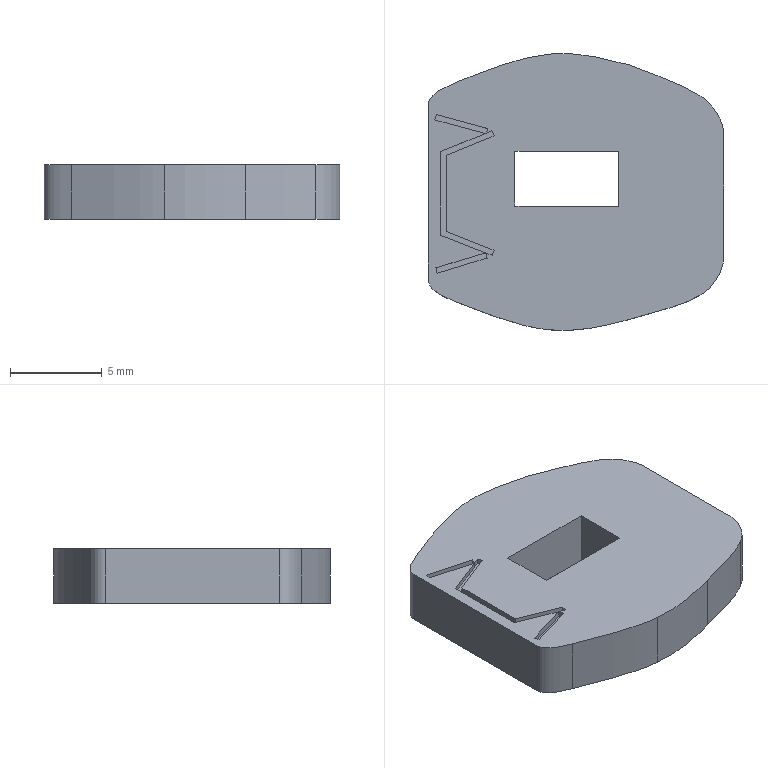Part | SolidWorks | features BaseBody 1 | 1 solid | 37 faces | box 16.136 x 15.14 x 3 mm | volume 585.362 mm3 | plane 26 | spline 11
STEP:
#1=CARTESIAN_POINT('',(-55.875,-105.115,1.2));
#2=VERTEX_POINT('',#1);
#3=CARTESIAN_POINT('',(-55.943,-105.364,1.2));
#4=VERTEX_POINT('',#3);
#5=CARTESIAN_POINT('',(-55.875,-105.115,1.2));
#6=DIRECTION('',(-0.2619,-0.9651,0.));
#7=VECTOR('',#6,1000.);
#8=LINE('',#5,#7);
#9=EDGE_CURVE('',#2,#4,#8,.T.);
#10=ORIENTED_EDGE('',*,*,#9,.F.);
#11=CARTESIAN_POINT('',(-58.677,-104.354,1.2));
#12=VERTEX_POINT('',#11);
#13=CARTESIAN_POINT('',(-55.875,-105.115,1.2));
#14=DIRECTION('',(-0.9651,0.2619,0.));
#15=VECTOR('',#14,1000.);
#16=LINE('',#13,#15);
#17=EDGE_CURVE('',#2,#12,#16,.T.);
#18=ORIENTED_EDGE('',*,*,#17,.T.);
#19=CARTESIAN_POINT('',(-58.755,-104.644,1.2));
#20=VERTEX_POINT('',#19);
#21=CARTESIAN_POINT('',(-58.755,-104.644,1.2));
#22=DIRECTION('',(0.2619,0.9651,0.));
#23=VECTOR('',#22,1000.);
#24=LINE('',#21,#23);
#25=EDGE_CURVE('',#20,#12,#24,.T.);
#26=ORIENTED_EDGE('',*,*,#25,.F.);
#27=CARTESIAN_POINT('',(-56.007,-105.39,1.2));
#28=VERTEX_POINT('',#27);
#29=CARTESIAN_POINT('',(-55.954,-105.404,1.2));
#30=DIRECTION('',(-0.9651,0.2619,0.));
#31=VECTOR('',#30,1000.);
#32=LINE('',#29,#31);
#33=EDGE_CURVE('',#28,#20,#32,.T.);
#34=ORIENTED_EDGE('',*,*,#33,.F.);
#35=CARTESIAN_POINT('',(-58.448,-106.374,1.2));
#36=VERTEX_POINT('',#35);
#37=CARTESIAN_POINT('',(-55.64,-105.242,1.2));
#38=DIRECTION('',(-0.9274,-0.3742,0.));
#39=VECTOR('',#38,1000.);
#40=LINE('',#37,#39);
#41=EDGE_CURVE('',#28,#36,#40,.T.);
#42=ORIENTED_EDGE('',*,*,#41,.T.);
#43=CARTESIAN_POINT('',(-58.448,-110.943,1.2));
#44=VERTEX_POINT('',#43);
#45=CARTESIAN_POINT('',(-58.448,-106.577,1.2));
#46=DIRECTION('',(0.,-1.,0.));
#47=VECTOR('',#46,1000.);
#48=LINE('',#45,#47);
#49=EDGE_CURVE('',#36,#44,#48,.T.);
#50=ORIENTED_EDGE('',*,*,#49,.T.);
#51=CARTESIAN_POINT('',(-55.637,-112.042,1.2));
#52=VERTEX_POINT('',#51);
#53=CARTESIAN_POINT('',(-58.257,-111.018,1.2));
#54=DIRECTION('',(0.9314,-0.3641,0.));
#55=VECTOR('',#54,1000.);
#56=LINE('',#53,#55);
#57=EDGE_CURVE('',#44,#52,#56,.T.);
#58=ORIENTED_EDGE('',*,*,#57,.T.);
#59=CARTESIAN_POINT('',(-55.528,-111.763,1.2));
#60=VERTEX_POINT('',#59);
#61=CARTESIAN_POINT('',(-55.528,-111.763,1.2));
#62=DIRECTION('',(-0.3641,-0.9314,0.));
#63=VECTOR('',#62,1000.);
#64=LINE('',#61,#63);
#65=EDGE_CURVE('',#60,#52,#64,.T.);
#66=ORIENTED_EDGE('',*,*,#65,.F.);
#67=CARTESIAN_POINT('',(-58.148,-110.738,1.2));
#68=VERTEX_POINT('',#67);
#69=CARTESIAN_POINT('',(-58.148,-110.738,1.2));
#70=DIRECTION('',(0.9314,-0.3641,0.));
#71=VECTOR('',#70,1000.);
#72=LINE('',#69,#71);
#73=EDGE_CURVE('',#68,#60,#72,.T.);
#74=ORIENTED_EDGE('',*,*,#73,.F.);
#75=CARTESIAN_POINT('',(-58.148,-106.577,1.2));
#76=VERTEX_POINT('',#75);
#77=CARTESIAN_POINT('',(-58.148,-106.577,1.2));
#78=DIRECTION('',(0.,-1.,0.));
#79=VECTOR('',#78,1000.);
#80=LINE('',#77,#79);
#81=EDGE_CURVE('',#76,#68,#80,.T.);
#82=ORIENTED_EDGE('',*,*,#81,.F.);
#83=CARTESIAN_POINT('',(-55.528,-105.52,1.2));
#84=VERTEX_POINT('',#83);
#85=CARTESIAN_POINT('',(-55.528,-105.52,1.2));
#86=DIRECTION('',(-0.9274,-0.3742,0.));
#87=VECTOR('',#86,1000.);
#88=LINE('',#85,#87);
#89=EDGE_CURVE('',#84,#76,#88,.T.);
#90=ORIENTED_EDGE('',*,*,#89,.F.);
#91=CARTESIAN_POINT('',(-55.64,-105.242,1.2));
#92=VERTEX_POINT('',#91);
#93=CARTESIAN_POINT('',(-55.64,-105.242,1.2));
#94=DIRECTION('',(0.3742,-0.9274,0.));
#95=VECTOR('',#94,1000.);
#96=LINE('',#93,#95);
#97=EDGE_CURVE('',#92,#84,#96,.T.);
#98=ORIENTED_EDGE('',*,*,#97,.F.);
#99=CARTESIAN_POINT('',(-55.64,-105.242,1.2));
#100=DIRECTION('',(-0.9274,-0.3742,0.));
#101=VECTOR('',#100,1000.);
#102=LINE('',#99,#101);
#103=EDGE_CURVE('',#92,#4,#102,.T.);
#104=ORIENTED_EDGE('',*,*,#103,.T.);
#105=EDGE_LOOP('',(#10,#18,#26,#34,#42,#50,#58,#66,#74,#82,#90,#98,#104));
#106=FACE_OUTER_BOUND('',#105,.T.);
#107=CARTESIAN_POINT('',(0.,0.,1.2));
#108=DIRECTION('',(0.,0.,-1.));
#109=DIRECTION('',(0.,-1.,0.));
#110=AXIS2_PLACEMENT_3D('',#107,#108,#109);
#111=PLANE('',#110);
#112=ADVANCED_FACE('',(#106),#111,.F.);
#113=CARTESIAN_POINT('',(-58.755,-104.644,1.5));
#114=VERTEX_POINT('',#113);
#115=CARTESIAN_POINT('',(-58.677,-104.354,1.5));
#116=VERTEX_POINT('',#115);
#117=CARTESIAN_POINT('',(-58.755,-104.644,1.5));
#118=DIRECTION('',(0.2619,0.9651,0.));
#119=VECTOR('',#118,1000.);
#120=LINE('',#117,#119);
#121=EDGE_CURVE('',#114,#116,#120,.T.);
#122=ORIENTED_EDGE('',*,*,#121,.F.);
#123=CARTESIAN_POINT('',(-58.755,-104.644,1.2));
#124=DIRECTION('',(0.,0.,1.));
#125=VECTOR('',#124,1000.);
#126=LINE('',#123,#125);
#127=EDGE_CURVE('',#20,#114,#126,.T.);
#128=ORIENTED_EDGE('',*,*,#127,.F.);
#129=ORIENTED_EDGE('',*,*,#25,.T.);
#130=CARTESIAN_POINT('',(-58.677,-104.354,1.2));
#131=DIRECTION('',(0.,0.,1.));
#132=VECTOR('',#131,1000.);
#133=LINE('',#130,#132);
#134=EDGE_CURVE('',#12,#116,#133,.T.);
#135=ORIENTED_EDGE('',*,*,#134,.T.);
#136=EDGE_LOOP('',(#122,#128,#129,#135));
#137=FACE_OUTER_BOUND('',#136,.T.);
#138=CARTESIAN_POINT('',(-58.755,-104.644,1.2));
#139=DIRECTION('',(0.9651,-0.2619,0.));
#140=DIRECTION('',(0.,0.,-1.));
#141=AXIS2_PLACEMENT_3D('',#138,#139,#140);
#142=PLANE('',#141);
#143=ADVANCED_FACE('',(#137),#142,.T.);
#144=CARTESIAN_POINT('',(-56.007,-105.39,1.5));
#145=VERTEX_POINT('',#144);
#146=CARTESIAN_POINT('',(-56.007,-105.39,1.2));
#147=DIRECTION('',(0.,0.,-1.));
#148=VECTOR('',#147,1000.);
#149=LINE('',#146,#148);
#150=EDGE_CURVE('',#145,#28,#149,.T.);
#151=ORIENTED_EDGE('',*,*,#150,.T.);
#152=ORIENTED_EDGE('',*,*,#33,.T.);
#153=ORIENTED_EDGE('',*,*,#127,.T.);
#154=CARTESIAN_POINT('',(-55.954,-105.404,1.5));
#155=DIRECTION('',(-0.9651,0.2619,0.));
#156=VECTOR('',#155,1000.);
#157=LINE('',#154,#156);
#158=EDGE_CURVE('',#145,#114,#157,.T.);
#159=ORIENTED_EDGE('',*,*,#158,.F.);
#160=EDGE_LOOP('',(#151,#152,#153,#159));
#161=FACE_OUTER_BOUND('',#160,.T.);
#162=CARTESIAN_POINT('',(-55.954,-105.404,1.2));
#163=DIRECTION('',(0.2619,0.9651,0.));
#164=DIRECTION('',(0.,0.,-1.));
#165=AXIS2_PLACEMENT_3D('',#162,#163,#164);
#166=PLANE('',#165);
#167=ADVANCED_FACE('',(#161),#166,.T.);
#168=CARTESIAN_POINT('',(-55.943,-105.364,1.5));
#169=VERTEX_POINT('',#168);
#170=CARTESIAN_POINT('',(-55.943,-105.364,1.2));
#171=DIRECTION('',(0.,0.,1.));
#172=VECTOR('',#171,1000.);
#173=LINE('',#170,#172);
#174=EDGE_CURVE('',#4,#169,#173,.T.);
#175=ORIENTED_EDGE('',*,*,#174,.T.);
#176=CARTESIAN_POINT('',(-55.875,-105.115,1.5));
#177=VERTEX_POINT('',#176);
#178=CARTESIAN_POINT('',(-55.875,-105.115,1.5));
#179=DIRECTION('',(-0.2619,-0.9651,0.));
#180=VECTOR('',#179,1000.);
#181=LINE('',#178,#180);
#182=EDGE_CURVE('',#177,#169,#181,.T.);
#183=ORIENTED_EDGE('',*,*,#182,.F.);
#184=CARTESIAN_POINT('',(-55.875,-105.115,1.2));
#185=DIRECTION('',(0.,0.,1.));
#186=VECTOR('',#185,1000.);
#187=LINE('',#184,#186);
#188=EDGE_CURVE('',#2,#177,#187,.T.);
#189=ORIENTED_EDGE('',*,*,#188,.F.);
#190=ORIENTED_EDGE('',*,*,#9,.T.);
#191=EDGE_LOOP('',(#175,#183,#189,#190));
#192=FACE_OUTER_BOUND('',#191,.T.);
#193=CARTESIAN_POINT('',(-55.875,-105.115,1.2));
#194=DIRECTION('',(-0.9651,0.2619,0.));
#195=DIRECTION('',(0.,0.,1.));
#196=AXIS2_PLACEMENT_3D('',#193,#194,#195);
#197=PLANE('',#196);
#198=ADVANCED_FACE('',(#192),#197,.T.);
#199=CARTESIAN_POINT('',(-55.875,-105.115,1.5));
#200=DIRECTION('',(-0.9651,0.2619,0.));
#201=VECTOR('',#200,1000.);
#202=LINE('',#199,#201);
#203=EDGE_CURVE('',#177,#116,#202,.T.);
#204=ORIENTED_EDGE('',*,*,#203,.T.);
#205=ORIENTED_EDGE('',*,*,#134,.F.);
#206=ORIENTED_EDGE('',*,*,#17,.F.);
#207=ORIENTED_EDGE('',*,*,#188,.T.);
#208=EDGE_LOOP('',(#204,#205,#206,#207));
#209=FACE_OUTER_BOUND('',#208,.T.);
#210=CARTESIAN_POINT('',(-55.875,-105.115,1.2));
#211=DIRECTION('',(0.2619,0.9651,0.));
#212=DIRECTION('',(0.,0.,-1.));
#213=AXIS2_PLACEMENT_3D('',#210,#211,#212);
#214=PLANE('',#213);
#215=ADVANCED_FACE('',(#209),#214,.F.);
#216=CARTESIAN_POINT('',(-58.448,-106.374,1.5));
#217=VERTEX_POINT('',#216);
#218=CARTESIAN_POINT('',(-55.64,-105.242,1.5));
#219=DIRECTION('',(-0.9274,-0.3742,0.));
#220=VECTOR('',#219,1000.);
#221=LINE('',#218,#220);
#222=EDGE_CURVE('',#145,#217,#221,.T.);
#223=ORIENTED_EDGE('',*,*,#222,.T.);
#224=CARTESIAN_POINT('',(-58.448,-106.374,1.2));
#225=DIRECTION('',(0.,0.,1.));
#226=VECTOR('',#225,1000.);
#227=LINE('',#224,#226);
#228=EDGE_CURVE('',#36,#217,#227,.T.);
#229=ORIENTED_EDGE('',*,*,#228,.F.);
#230=ORIENTED_EDGE('',*,*,#41,.F.);
#231=ORIENTED_EDGE('',*,*,#150,.F.);
#232=EDGE_LOOP('',(#223,#229,#230,#231));
#233=FACE_OUTER_BOUND('',#232,.T.);
#234=CARTESIAN_POINT('',(-55.64,-105.242,1.2));
#235=DIRECTION('',(-0.3742,0.9274,0.));
#236=DIRECTION('',(0.,0.,1.));
#237=AXIS2_PLACEMENT_3D('',#234,#235,#236);
#238=PLANE('',#237);
#239=ADVANCED_FACE('',(#233),#238,.F.);
#240=CARTESIAN_POINT('',(-58.448,-110.943,1.5));
#241=VERTEX_POINT('',#240);
#242=CARTESIAN_POINT('',(-58.448,-106.577,1.5));
#243=DIRECTION('',(0.,-1.,0.));
#244=VECTOR('',#243,1000.);
#245=LINE('',#242,#244);
#246=EDGE_CURVE('',#217,#241,#245,.T.);
#247=ORIENTED_EDGE('',*,*,#246,.T.);
#248=CARTESIAN_POINT('',(-58.448,-110.943,1.2));
#249=DIRECTION('',(0.,0.,1.));
#250=VECTOR('',#249,1000.);
#251=LINE('',#248,#250);
#252=EDGE_CURVE('',#44,#241,#251,.T.);
#253=ORIENTED_EDGE('',*,*,#252,.F.);
#254=ORIENTED_EDGE('',*,*,#49,.F.);
#255=ORIENTED_EDGE('',*,*,#228,.T.);
#256=EDGE_LOOP('',(#247,#253,#254,#255));
#257=FACE_OUTER_BOUND('',#256,.T.);
#258=CARTESIAN_POINT('',(-58.448,-106.577,1.2));
#259=DIRECTION('',(-1.,0.,0.));
#260=DIRECTION('',(0.,0.,1.));
#261=AXIS2_PLACEMENT_3D('',#258,#259,#260);
#262=PLANE('',#261);
#263=ADVANCED_FACE('',(#257),#262,.F.);
#264=CARTESIAN_POINT('',(-55.637,-112.042,1.5));
#265=VERTEX_POINT('',#264);
#266=CARTESIAN_POINT('',(-58.257,-111.018,1.5));
#267=DIRECTION('',(0.9314,-0.3641,0.));
#268=VECTOR('',#267,1000.);
#269=LINE('',#266,#268);
#270=EDGE_CURVE('',#241,#265,#269,.T.);
#271=ORIENTED_EDGE('',*,*,#270,.T.);
#272=CARTESIAN_POINT('',(-55.637,-112.042,1.2));
#273=DIRECTION('',(0.,0.,1.));
#274=VECTOR('',#273,1000.);
#275=LINE('',#272,#274);
#276=EDGE_CURVE('',#52,#265,#275,.T.);
#277=ORIENTED_EDGE('',*,*,#276,.F.);
#278=ORIENTED_EDGE('',*,*,#57,.F.);
#279=ORIENTED_EDGE('',*,*,#252,.T.);
#280=EDGE_LOOP('',(#271,#277,#278,#279));
#281=FACE_OUTER_BOUND('',#280,.T.);
#282=CARTESIAN_POINT('',(-58.257,-111.018,1.2));
#283=DIRECTION('',(-0.3641,-0.9314,0.));
#284=DIRECTION('',(-0.9314,0.3641,0.));
#285=AXIS2_PLACEMENT_3D('',#282,#283,#284);
#286=PLANE('',#285);
#287=ADVANCED_FACE('',(#281),#286,.F.);
#288=CARTESIAN_POINT('',(-55.528,-111.763,1.5));
#289=VERTEX_POINT('',#288);
#290=CARTESIAN_POINT('',(-55.528,-111.763,1.5));
#291=DIRECTION('',(-0.3641,-0.9314,0.));
#292=VECTOR('',#291,1000.);
#293=LINE('',#290,#292);
#294=EDGE_CURVE('',#289,#265,#293,.T.);
#295=ORIENTED_EDGE('',*,*,#294,.F.);
#296=CARTESIAN_POINT('',(-55.528,-111.763,1.2));
#297=DIRECTION('',(0.,0.,1.));
#298=VECTOR('',#297,1000.);
#299=LINE('',#296,#298);
#300=EDGE_CURVE('',#60,#289,#299,.T.);
#301=ORIENTED_EDGE('',*,*,#300,.F.);
#302=ORIENTED_EDGE('',*,*,#65,.T.);
#303=ORIENTED_EDGE('',*,*,#276,.T.);
#304=EDGE_LOOP('',(#295,#301,#302,#303));
#305=FACE_OUTER_BOUND('',#304,.T.);
#306=CARTESIAN_POINT('',(-55.528,-111.763,1.2));
#307=DIRECTION('',(-0.9314,0.3641,0.));
#308=DIRECTION('',(0.,0.,1.));
#309=AXIS2_PLACEMENT_3D('',#306,#307,#308);
#310=PLANE('',#309);
#311=ADVANCED_FACE('',(#305),#310,.T.);
#312=CARTESIAN_POINT('',(-58.148,-110.738,1.5));
#313=VERTEX_POINT('',#312);
#314=CARTESIAN_POINT('',(-58.148,-110.738,1.5));
#315=DIRECTION('',(0.9314,-0.3641,0.));
#316=VECTOR('',#315,1000.);
#317=LINE('',#314,#316);
#318=EDGE_CURVE('',#313,#289,#317,.T.);
#319=ORIENTED_EDGE('',*,*,#318,.F.);
#320=CARTESIAN_POINT('',(-58.148,-110.738,1.2));
#321=DIRECTION('',(0.,0.,1.));
#322=VECTOR('',#321,1000.);
#323=LINE('',#320,#322);
#324=EDGE_CURVE('',#68,#313,#323,.T.);
#325=ORIENTED_EDGE('',*,*,#324,.F.);
#326=ORIENTED_EDGE('',*,*,#73,.T.);
#327=ORIENTED_EDGE('',*,*,#300,.T.);
#328=EDGE_LOOP('',(#319,#325,#326,#327));
#329=FACE_OUTER_BOUND('',#328,.T.);
#330=CARTESIAN_POINT('',(-58.148,-110.738,1.2));
#331=DIRECTION('',(-0.3641,-0.9314,0.));
#332=DIRECTION('',(-0.9314,0.3641,0.));
#333=AXIS2_PLACEMENT_3D('',#330,#331,#332);
#334=PLANE('',#333);
#335=ADVANCED_FACE('',(#329),#334,.T.);
#336=CARTESIAN_POINT('',(-58.148,-106.577,1.5));
#337=VERTEX_POINT('',#336);
#338=CARTESIAN_POINT('',(-58.148,-106.577,1.5));
#339=DIRECTION('',(0.,-1.,0.));
#340=VECTOR('',#339,1000.);
#341=LINE('',#338,#340);
#342=EDGE_CURVE('',#337,#313,#341,.T.);
#343=ORIENTED_EDGE('',*,*,#342,.F.);
#344=CARTESIAN_POINT('',(-58.148,-106.577,1.2));
#345=DIRECTION('',(0.,0.,1.));
#346=VECTOR('',#345,1000.);
#347=LINE('',#344,#346);
#348=EDGE_CURVE('',#76,#337,#347,.T.);
#349=ORIENTED_EDGE('',*,*,#348,.F.);
#350=ORIENTED_EDGE('',*,*,#81,.T.);
#351=ORIENTED_EDGE('',*,*,#324,.T.);
#352=EDGE_LOOP('',(#343,#349,#350,#351));
#353=FACE_OUTER_BOUND('',#352,.T.);
#354=CARTESIAN_POINT('',(-58.148,-106.577,1.2));
#355=DIRECTION('',(-1.,0.,0.));
#356=DIRECTION('',(0.,0.,1.));
#357=AXIS2_PLACEMENT_3D('',#354,#355,#356);
#358=PLANE('',#357);
#359=ADVANCED_FACE('',(#353),#358,.T.);
#360=CARTESIAN_POINT('',(-55.528,-105.52,1.5));
#361=VERTEX_POINT('',#360);
#362=CARTESIAN_POINT('',(-55.528,-105.52,1.5));
#363=DIRECTION('',(-0.9274,-0.3742,0.));
#364=VECTOR('',#363,1000.);
#365=LINE('',#362,#364);
#366=EDGE_CURVE('',#361,#337,#365,.T.);
#367=ORIENTED_EDGE('',*,*,#366,.F.);
#368=CARTESIAN_POINT('',(-55.528,-105.52,1.2));
#369=DIRECTION('',(0.,0.,1.));
#370=VECTOR('',#369,1000.);
#371=LINE('',#368,#370);
#372=EDGE_CURVE('',#84,#361,#371,.T.);
#373=ORIENTED_EDGE('',*,*,#372,.F.);
#374=ORIENTED_EDGE('',*,*,#89,.T.);
#375=ORIENTED_EDGE('',*,*,#348,.T.);
#376=EDGE_LOOP('',(#367,#373,#374,#375));
#377=FACE_OUTER_BOUND('',#376,.T.);
#378=CARTESIAN_POINT('',(-55.528,-105.52,1.2));
#379=DIRECTION('',(-0.3742,0.9274,0.));
#380=DIRECTION('',(0.,0.,1.));
#381=AXIS2_PLACEMENT_3D('',#378,#379,#380);
#382=PLANE('',#381);
#383=ADVANCED_FACE('',(#377),#382,.T.);
#384=CARTESIAN_POINT('',(-55.64,-105.242,1.5));
#385=VERTEX_POINT('',#384);
#386=CARTESIAN_POINT('',(-55.64,-105.242,1.5));
#387=DIRECTION('',(0.3742,-0.9274,0.));
#388=VECTOR('',#387,1000.);
#389=LINE('',#386,#388);
#390=EDGE_CURVE('',#385,#361,#389,.T.);
#391=ORIENTED_EDGE('',*,*,#390,.F.);
#392=CARTESIAN_POINT('',(-55.64,-105.242,1.2));
#393=DIRECTION('',(0.,0.,1.));
#394=VECTOR('',#393,1000.);
#395=LINE('',#392,#394);
#396=EDGE_CURVE('',#92,#385,#395,.T.);
#397=ORIENTED_EDGE('',*,*,#396,.F.);
#398=ORIENTED_EDGE('',*,*,#97,.T.);
#399=ORIENTED_EDGE('',*,*,#372,.T.);
#400=EDGE_LOOP('',(#391,#397,#398,#399));
#401=FACE_OUTER_BOUND('',#400,.T.);
#402=CARTESIAN_POINT('',(-55.64,-105.242,1.2));
#403=DIRECTION('',(-0.9274,-0.3742,0.));
#404=DIRECTION('',(-0.3742,0.9274,0.));
#405=AXIS2_PLACEMENT_3D('',#402,#403,#404);
#406=PLANE('',#405);
#407=ADVANCED_FACE('',(#401),#406,.T.);
#408=ORIENTED_EDGE('',*,*,#103,.F.);
#409=ORIENTED_EDGE('',*,*,#396,.T.);
#410=CARTESIAN_POINT('',(-55.64,-105.242,1.5));
#411=DIRECTION('',(-0.9274,-0.3742,0.));
#412=VECTOR('',#411,1000.);
#413=LINE('',#410,#412);
#414=EDGE_CURVE('',#385,#169,#413,.T.);
#415=ORIENTED_EDGE('',*,*,#414,.T.);
#416=ORIENTED_EDGE('',*,*,#174,.F.);
#417=EDGE_LOOP('',(#408,#409,#415,#416));
#418=FACE_OUTER_BOUND('',#417,.T.);
#419=CARTESIAN_POINT('',(-55.64,-105.242,1.2));
#420=DIRECTION('',(-0.3742,0.9274,0.));
#421=DIRECTION('',(0.,0.,1.));
#422=AXIS2_PLACEMENT_3D('',#419,#420,#421);
#423=PLANE('',#422);
#424=ADVANCED_FACE('',(#418),#423,.F.);
#425=CARTESIAN_POINT('',(-58.627,-113.019,1.2));
#426=VERTEX_POINT('',#425);
#427=CARTESIAN_POINT('',(-55.905,-112.191,1.2));
#428=VERTEX_POINT('',#427);
#429=CARTESIAN_POINT('',(-58.627,-113.019,1.2));
#430=DIRECTION('',(0.9567,0.2911,0.));
#431=VECTOR('',#430,1000.);
#432=LINE('',#429,#431);
#433=EDGE_CURVE('',#426,#428,#432,.T.);
#434=ORIENTED_EDGE('',*,*,#433,.T.);
#435=CARTESIAN_POINT('',(-55.992,-111.904,1.2));
#436=VERTEX_POINT('',#435);
#437=CARTESIAN_POINT('',(-55.992,-111.904,1.2));
#438=DIRECTION('',(0.2911,-0.9567,0.));
#439=VECTOR('',#438,1000.);
#440=LINE('',#437,#439);
#441=EDGE_CURVE('',#436,#428,#440,.T.);
#442=ORIENTED_EDGE('',*,*,#441,.F.);
#443=CARTESIAN_POINT('',(-58.714,-112.732,1.2));
#444=VERTEX_POINT('',#443);
#445=CARTESIAN_POINT('',(-58.714,-112.732,1.2));
#446=DIRECTION('',(0.9567,0.2911,0.));
#447=VECTOR('',#446,1000.);
#448=LINE('',#445,#447);
#449=EDGE_CURVE('',#444,#436,#448,.T.);
#450=ORIENTED_EDGE('',*,*,#449,.F.);
#451=CARTESIAN_POINT('',(-58.627,-113.019,1.2));
#452=DIRECTION('',(-0.2911,0.9567,0.));
#453=VECTOR('',#452,1000.);
#454=LINE('',#451,#453);
#455=EDGE_CURVE('',#426,#444,#454,.T.);
#456=ORIENTED_EDGE('',*,*,#455,.F.);
#457=EDGE_LOOP('',(#434,#442,#450,#456));
#458=FACE_OUTER_BOUND('',#457,.T.);
#459=CARTESIAN_POINT('',(0.,0.,1.2));
#460=DIRECTION('',(0.,0.,-1.));
#461=DIRECTION('',(0.,-1.,0.));
#462=AXIS2_PLACEMENT_3D('',#459,#460,#461);
#463=PLANE('',#462);
#464=ADVANCED_FACE('',(#458),#463,.F.);
#465=CARTESIAN_POINT('',(-55.992,-111.904,1.5));
#466=VERTEX_POINT('',#465);
#467=CARTESIAN_POINT('',(-55.905,-112.191,1.5));
#468=VERTEX_POINT('',#467);
#469=CARTESIAN_POINT('',(-55.992,-111.904,1.5));
#470=DIRECTION('',(0.2911,-0.9567,0.));
#471=VECTOR('',#470,1000.);
#472=LINE('',#469,#471);
#473=EDGE_CURVE('',#466,#468,#472,.T.);
#474=ORIENTED_EDGE('',*,*,#473,.F.);
#475=CARTESIAN_POINT('',(-55.992,-111.904,1.2));
#476=DIRECTION('',(0.,0.,1.));
#477=VECTOR('',#476,1000.);
#478=LINE('',#475,#477);
#479=EDGE_CURVE('',#436,#466,#478,.T.);
#480=ORIENTED_EDGE('',*,*,#479,.F.);
#481=ORIENTED_EDGE('',*,*,#441,.T.);
#482=CARTESIAN_POINT('',(-55.905,-112.191,1.2));
#483=DIRECTION('',(0.,0.,1.));
#484=VECTOR('',#483,1000.);
#485=LINE('',#482,#484);
#486=EDGE_CURVE('',#428,#468,#485,.T.);
#487=ORIENTED_EDGE('',*,*,#486,.T.);
#488=EDGE_LOOP('',(#474,#480,#481,#487));
#489=FACE_OUTER_BOUND('',#488,.T.);
#490=CARTESIAN_POINT('',(-55.992,-111.904,1.2));
#491=DIRECTION('',(-0.9567,-0.2911,0.));
#492=DIRECTION('',(-0.2911,0.9567,0.));
#493=AXIS2_PLACEMENT_3D('',#490,#491,#492);
#494=PLANE('',#493);
#495=ADVANCED_FACE('',(#489),#494,.T.);
#496=CARTESIAN_POINT('',(-58.714,-112.732,1.5));
#497=VERTEX_POINT('',#496);
#498=CARTESIAN_POINT('',(-58.714,-112.732,1.5));
#499=DIRECTION('',(0.9567,0.2911,0.));
#500=VECTOR('',#499,1000.);
#501=LINE('',#498,#500);
#502=EDGE_CURVE('',#497,#466,#501,.T.);
#503=ORIENTED_EDGE('',*,*,#502,.F.);
#504=CARTESIAN_POINT('',(-58.714,-112.732,1.2));
#505=DIRECTION('',(0.,0.,1.));
#506=VECTOR('',#505,1000.);
#507=LINE('',#504,#506);
#508=EDGE_CURVE('',#444,#497,#507,.T.);
#509=ORIENTED_EDGE('',*,*,#508,.F.);
#510=ORIENTED_EDGE('',*,*,#449,.T.);
#511=ORIENTED_EDGE('',*,*,#479,.T.);
#512=EDGE_LOOP('',(#503,#509,#510,#511));
#513=FACE_OUTER_BOUND('',#512,.T.);
#514=CARTESIAN_POINT('',(-58.714,-112.732,1.2));
#515=DIRECTION('',(0.2911,-0.9567,0.));
#516=DIRECTION('',(0.,0.,-1.));
#517=AXIS2_PLACEMENT_3D('',#514,#515,#516);
#518=PLANE('',#517);
#519=ADVANCED_FACE('',(#513),#518,.T.);
#520=CARTESIAN_POINT('',(-58.627,-113.019,1.5));
#521=VERTEX_POINT('',#520);
#522=CARTESIAN_POINT('',(-58.627,-113.019,1.5));
#523=DIRECTION('',(-0.2911,0.9567,0.));
#524=VECTOR('',#523,1000.);
#525=LINE('',#522,#524);
#526=EDGE_CURVE('',#521,#497,#525,.T.);
#527=ORIENTED_EDGE('',*,*,#526,.F.);
#528=CARTESIAN_POINT('',(-58.627,-113.019,1.2));
#529=DIRECTION('',(0.,0.,1.));
#530=VECTOR('',#529,1000.);
#531=LINE('',#528,#530);
#532=EDGE_CURVE('',#426,#521,#531,.T.);
#533=ORIENTED_EDGE('',*,*,#532,.F.);
#534=ORIENTED_EDGE('',*,*,#455,.T.);
#535=ORIENTED_EDGE('',*,*,#508,.T.);
#536=EDGE_LOOP('',(#527,#533,#534,#535));
#537=FACE_OUTER_BOUND('',#536,.T.);
#538=CARTESIAN_POINT('',(-58.627,-113.019,1.2));
#539=DIRECTION('',(0.9567,0.2911,0.));
#540=DIRECTION('',(0.,0.,-1.));
#541=AXIS2_PLACEMENT_3D('',#538,#539,#540);
#542=PLANE('',#541);
#543=ADVANCED_FACE('',(#537),#542,.T.);
#544=CARTESIAN_POINT('',(-58.627,-113.019,1.5));
#545=DIRECTION('',(0.9567,0.2911,0.));
#546=VECTOR('',#545,1000.);
#547=LINE('',#544,#546);
#548=EDGE_CURVE('',#521,#468,#547,.T.);
#549=ORIENTED_EDGE('',*,*,#548,.T.);
#550=ORIENTED_EDGE('',*,*,#486,.F.);
#551=ORIENTED_EDGE('',*,*,#433,.F.);
#552=ORIENTED_EDGE('',*,*,#532,.T.);
#553=EDGE_LOOP('',(#549,#550,#551,#552));
#554=FACE_OUTER_BOUND('',#553,.T.);
#555=CARTESIAN_POINT('',(-58.627,-113.019,1.2));
#556=DIRECTION('',(0.2911,-0.9567,0.));
#557=DIRECTION('',(0.,0.,-1.));
#558=AXIS2_PLACEMENT_3D('',#555,#556,#557);
#559=PLANE('',#558);
#560=ADVANCED_FACE('',(#554),#559,.F.);
#561=CARTESIAN_POINT('',(-54.383,-106.352,1.5));
#562=VERTEX_POINT('',#561);
#563=CARTESIAN_POINT('',(-54.383,-109.349,1.5));
#564=VERTEX_POINT('',#563);
#565=CARTESIAN_POINT('',(-54.383,0.,1.5));
#566=DIRECTION('',(0.,-1.,0.));
#567=VECTOR('',#566,1000.);
#568=LINE('',#565,#567);
#569=EDGE_CURVE('',#562,#564,#568,.T.);
#570=ORIENTED_EDGE('',*,*,#569,.F.);
#571=CARTESIAN_POINT('',(-48.716,-106.352,1.5));
#572=VERTEX_POINT('',#571);
#573=CARTESIAN_POINT('',(0.,-106.352,1.5));
#574=DIRECTION('',(-1.,0.,0.));
#575=VECTOR('',#574,1000.);
#576=LINE('',#573,#575);
#577=EDGE_CURVE('',#572,#562,#576,.T.);
#578=ORIENTED_EDGE('',*,*,#577,.F.);
#579=CARTESIAN_POINT('',(-48.716,-109.349,1.5));
#580=VERTEX_POINT('',#579);
#581=CARTESIAN_POINT('',(-48.716,0.,1.5));
#582=DIRECTION('',(0.,1.,0.));
#583=VECTOR('',#582,1000.);
#584=LINE('',#581,#583);
#585=EDGE_CURVE('',#580,#572,#584,.T.);
#586=ORIENTED_EDGE('',*,*,#585,.F.);
#587=CARTESIAN_POINT('',(0.,-109.349,1.5));
#588=DIRECTION('',(1.,0.,0.));
#589=VECTOR('',#588,1000.);
#590=LINE('',#587,#589);
#591=EDGE_CURVE('',#564,#580,#590,.T.);
#592=ORIENTED_EDGE('',*,*,#591,.F.);
#593=EDGE_LOOP('',(#570,#578,#586,#592));
#594=FACE_BOUND('',#593,.T.);
#595=ORIENTED_EDGE('',*,*,#548,.F.);
#596=ORIENTED_EDGE('',*,*,#526,.T.);
#597=ORIENTED_EDGE('',*,*,#502,.T.);
#598=ORIENTED_EDGE('',*,*,#473,.T.);
#599=EDGE_LOOP('',(#595,#596,#597,#598));
#600=FACE_BOUND('',#599,.T.);
#601=ORIENTED_EDGE('',*,*,#414,.F.);
#602=ORIENTED_EDGE('',*,*,#390,.T.);
#603=ORIENTED_EDGE('',*,*,#366,.T.);
#604=ORIENTED_EDGE('',*,*,#342,.T.);
#605=ORIENTED_EDGE('',*,*,#318,.T.);
#606=ORIENTED_EDGE('',*,*,#294,.T.);
#607=ORIENTED_EDGE('',*,*,#270,.F.);
#608=ORIENTED_EDGE('',*,*,#246,.F.);
#609=ORIENTED_EDGE('',*,*,#222,.F.);
#610=ORIENTED_EDGE('',*,*,#158,.T.);
#611=ORIENTED_EDGE('',*,*,#121,.T.);
#612=ORIENTED_EDGE('',*,*,#203,.F.);
#613=ORIENTED_EDGE('',*,*,#182,.T.);
#614=EDGE_LOOP('',(#601,#602,#603,#604,#605,#606,#607,#608,#609,#610,#611,#612,#613));
#615=FACE_BOUND('',#614,.T.);
#616=CARTESIAN_POINT('',(-52.548,-101.05,1.5));
#617=VERTEX_POINT('',#616);
#618=CARTESIAN_POINT('',(-57.632,-102.605,1.5));
#619=VERTEX_POINT('',#618);
#620=CARTESIAN_POINT('',(-52.548,-101.05,1.5));
#621=CARTESIAN_POINT('',(-54.13,-101.211,1.5));
#622=CARTESIAN_POINT('',(-55.88,-101.908,1.5));
#623=CARTESIAN_POINT('',(-57.632,-102.605,1.5));
#624=B_SPLINE_CURVE_WITH_KNOTS('',3,(#620,#621,#622,#623),.UNSPECIFIED.,.F.,.F.,(4,4),(0.3913,0.4348),.UNSPECIFIED.);
#625=EDGE_CURVE('',#617,#619,#624,.T.);
#626=ORIENTED_EDGE('',*,*,#625,.T.);
#627=CARTESIAN_POINT('',(-59.117,-103.845,1.5));
#628=VERTEX_POINT('',#627);
#629=CARTESIAN_POINT('',(-57.632,-102.605,1.5));
#630=CARTESIAN_POINT('',(-58.373,-102.911,1.5));
#631=CARTESIAN_POINT('',(-59.117,-103.219,1.5));
#632=CARTESIAN_POINT('',(-59.117,-103.845,1.5));
#633=B_SPLINE_CURVE_WITH_KNOTS('',3,(#629,#630,#631,#632),.UNSPECIFIED.,.F.,.F.,(4,4),(0.4348,0.4783),.UNSPECIFIED.);
#634=EDGE_CURVE('',#619,#628,#633,.T.);
#635=ORIENTED_EDGE('',*,*,#634,.T.);
#636=CARTESIAN_POINT('',(-59.117,-113.34,1.5));
#637=VERTEX_POINT('',#636);
#638=CARTESIAN_POINT('',(-59.117,0.,1.5));
#639=DIRECTION('',(0.,-1.,0.));
#640=VECTOR('',#639,1000.);
#641=LINE('',#638,#640);
#642=EDGE_CURVE('',#628,#637,#641,.T.);
#643=ORIENTED_EDGE('',*,*,#642,.T.);
#644=CARTESIAN_POINT('',(-57.632,-114.577,1.5));
#645=VERTEX_POINT('',#644);
#646=CARTESIAN_POINT('',(-59.117,-113.34,1.5));
#647=CARTESIAN_POINT('',(-59.117,-113.963,1.5));
#648=CARTESIAN_POINT('',(-58.373,-114.27,1.5));
#649=CARTESIAN_POINT('',(-57.632,-114.577,1.5));
#650=B_SPLINE_CURVE_WITH_KNOTS('',3,(#646,#647,#648,#649),.UNSPECIFIED.,.F.,.F.,(4,4),(0.,0.04348),.UNSPECIFIED.);
#651=EDGE_CURVE('',#637,#645,#650,.T.);
#652=ORIENTED_EDGE('',*,*,#651,.T.);
#653=CARTESIAN_POINT('',(-52.548,-116.113,1.5));
#654=VERTEX_POINT('',#653);
#655=CARTESIAN_POINT('',(-57.632,-114.577,1.5));
#656=CARTESIAN_POINT('',(-55.88,-115.264,1.5));
#657=CARTESIAN_POINT('',(-54.13,-115.952,1.5));
#658=CARTESIAN_POINT('',(-52.548,-116.113,1.5));
#659=B_SPLINE_CURVE_WITH_KNOTS('',3,(#655,#656,#657,#658),.UNSPECIFIED.,.F.,.F.,(4,4),(0.04348,0.08696),.UNSPECIFIED.);
#660=EDGE_CURVE('',#645,#654,#659,.T.);
#661=ORIENTED_EDGE('',*,*,#660,.T.);
#662=CARTESIAN_POINT('',(-48.141,-115.545,1.5));
#663=VERTEX_POINT('',#662);
#664=CARTESIAN_POINT('',(-52.548,-116.113,1.5));
#665=CARTESIAN_POINT('',(-50.967,-116.274,1.5));
#666=CARTESIAN_POINT('',(-49.553,-115.911,1.5));
#667=CARTESIAN_POINT('',(-48.141,-115.545,1.5));
#668=B_SPLINE_CURVE_WITH_KNOTS('',3,(#664,#665,#666,#667),.UNSPECIFIED.,.F.,.F.,(4,4),(0.08696,0.1304),.UNSPECIFIED.);
#669=EDGE_CURVE('',#654,#663,#668,.T.);
#670=ORIENTED_EDGE('',*,*,#669,.T.);
#671=CARTESIAN_POINT('',(-44.275,-114.232,1.5));
#672=VERTEX_POINT('',#671);
#673=CARTESIAN_POINT('',(-48.141,-115.545,1.5));
#674=CARTESIAN_POINT('',(-46.639,-115.139,1.5));
#675=CARTESIAN_POINT('',(-45.135,-114.736,1.5));
#676=CARTESIAN_POINT('',(-44.275,-114.232,1.5));
#677=B_SPLINE_CURVE_WITH_KNOTS('',3,(#673,#674,#675,#676),.UNSPECIFIED.,.F.,.F.,(4,4),(0.1304,0.1739),.UNSPECIFIED.);
#678=EDGE_CURVE('',#663,#672,#677,.T.);
#679=ORIENTED_EDGE('',*,*,#678,.T.);
#680=CARTESIAN_POINT('',(-42.981,-112.2,1.5));
#681=VERTEX_POINT('',#680);
#682=CARTESIAN_POINT('',(-44.275,-114.232,1.5));
#683=CARTESIAN_POINT('',(-43.416,-113.731,1.5));
#684=CARTESIAN_POINT('',(-42.981,-112.745,1.5));
#685=CARTESIAN_POINT('',(-42.981,-112.2,1.5));
#686=B_SPLINE_CURVE_WITH_KNOTS('',3,(#682,#683,#684,#685),.UNSPECIFIED.,.F.,.F.,(4,4),(0.1739,0.2174),.UNSPECIFIED.);
#687=EDGE_CURVE('',#672,#681,#686,.T.);
#688=ORIENTED_EDGE('',*,*,#687,.T.);
#689=CARTESIAN_POINT('',(-42.981,-105.35,1.5));
#690=VERTEX_POINT('',#689);
#691=CARTESIAN_POINT('',(-42.981,-112.2,1.5));
#692=CARTESIAN_POINT('',(-42.98,-110.022,1.5));
#693=CARTESIAN_POINT('',(-42.981,-107.632,1.5));
#694=CARTESIAN_POINT('',(-42.981,-105.35,1.5));
#695=B_SPLINE_CURVE_WITH_KNOTS('',3,(#691,#692,#693,#694),.UNSPECIFIED.,.F.,.F.,(4,4),(0.2174,0.2609),.UNSPECIFIED.);
#696=EDGE_CURVE('',#681,#690,#695,.T.);
#697=ORIENTED_EDGE('',*,*,#696,.T.);
#698=CARTESIAN_POINT('',(-44.275,-103.318,1.5));
#699=VERTEX_POINT('',#698);
#700=CARTESIAN_POINT('',(-42.981,-105.35,1.5));
#701=CARTESIAN_POINT('',(-42.981,-104.805,1.5));
#702=CARTESIAN_POINT('',(-43.416,-103.881,1.5));
#703=CARTESIAN_POINT('',(-44.275,-103.318,1.5));
#704=B_SPLINE_CURVE_WITH_KNOTS('',3,(#700,#701,#702,#703),.UNSPECIFIED.,.F.,.F.,(4,4),(0.2609,0.3043),.UNSPECIFIED.);
#705=EDGE_CURVE('',#690,#699,#704,.T.);
#706=ORIENTED_EDGE('',*,*,#705,.T.);
#707=CARTESIAN_POINT('',(-48.141,-101.641,1.5));
#708=VERTEX_POINT('',#707);
#709=CARTESIAN_POINT('',(-44.275,-103.318,1.5));
#710=CARTESIAN_POINT('',(-45.135,-102.755,1.5));
#711=CARTESIAN_POINT('',(-46.639,-102.197,1.5));
#712=CARTESIAN_POINT('',(-48.141,-101.641,1.5));
#713=B_SPLINE_CURVE_WITH_KNOTS('',3,(#709,#710,#711,#712),.UNSPECIFIED.,.F.,.F.,(4,4),(0.3043,0.3478),.UNSPECIFIED.);
#714=EDGE_CURVE('',#699,#708,#713,.T.);
#715=ORIENTED_EDGE('',*,*,#714,.T.);
#716=CARTESIAN_POINT('',(-48.141,-101.641,1.5));
#717=CARTESIAN_POINT('',(-49.553,-101.265,1.5));
#718=CARTESIAN_POINT('',(-50.965,-100.891,1.5));
#719=CARTESIAN_POINT('',(-52.548,-101.05,1.5));
#720=B_SPLINE_CURVE_WITH_KNOTS('',3,(#716,#717,#718,#719),.UNSPECIFIED.,.F.,.F.,(4,4),(0.3478,0.3913),.UNSPECIFIED.);
#721=EDGE_CURVE('',#708,#617,#720,.T.);
#722=ORIENTED_EDGE('',*,*,#721,.T.);
#723=EDGE_LOOP('',(#626,#635,#643,#652,#661,#670,#679,#688,#697,#706,#715,#722));
#724=FACE_OUTER_BOUND('',#723,.T.);
#725=CARTESIAN_POINT('',(0.,0.,1.5));
#726=DIRECTION('',(0.,0.,1.));
#727=DIRECTION('',(1.,0.,0.));
#728=AXIS2_PLACEMENT_3D('',#725,#726,#727);
#729=PLANE('',#728);
#730=ADVANCED_FACE('',(#594,#600,#615,#724),#729,.T.);
#731=CARTESIAN_POINT('',(-54.383,-106.352,-1.5));
#732=VERTEX_POINT('',#731);
#733=CARTESIAN_POINT('',(-54.383,-109.349,-1.5));
#734=VERTEX_POINT('',#733);
#735=CARTESIAN_POINT('',(-54.383,0.,-1.5));
#736=DIRECTION('',(0.,-1.,0.));
#737=VECTOR('',#736,1000.);
#738=LINE('',#735,#737);
#739=EDGE_CURVE('',#732,#734,#738,.T.);
#740=ORIENTED_EDGE('',*,*,#739,.T.);
#741=CARTESIAN_POINT('',(-48.716,-109.349,-1.5));
#742=VERTEX_POINT('',#741);
#743=CARTESIAN_POINT('',(0.,-109.349,-1.5));
#744=DIRECTION('',(1.,0.,0.));
#745=VECTOR('',#744,1000.);
#746=LINE('',#743,#745);
#747=EDGE_CURVE('',#734,#742,#746,.T.);
#748=ORIENTED_EDGE('',*,*,#747,.T.);
#749=CARTESIAN_POINT('',(-48.716,-106.352,-1.5));
#750=VERTEX_POINT('',#749);
#751=CARTESIAN_POINT('',(-48.716,0.,-1.5));
#752=DIRECTION('',(0.,1.,0.));
#753=VECTOR('',#752,1000.);
#754=LINE('',#751,#753);
#755=EDGE_CURVE('',#742,#750,#754,.T.);
#756=ORIENTED_EDGE('',*,*,#755,.T.);
#757=CARTESIAN_POINT('',(0.,-106.352,-1.5));
#758=DIRECTION('',(-1.,0.,0.));
#759=VECTOR('',#758,1000.);
#760=LINE('',#757,#759);
#761=EDGE_CURVE('',#750,#732,#760,.T.);
#762=ORIENTED_EDGE('',*,*,#761,.T.);
#763=EDGE_LOOP('',(#740,#748,#756,#762));
#764=FACE_BOUND('',#763,.T.);
#765=CARTESIAN_POINT('',(-52.548,-101.05,-1.5));
#766=VERTEX_POINT('',#765);
#767=CARTESIAN_POINT('',(-57.632,-102.605,-1.5));
#768=VERTEX_POINT('',#767);
#769=CARTESIAN_POINT('',(-52.548,-101.05,-1.5));
#770=CARTESIAN_POINT('',(-54.13,-101.211,-1.5));
#771=CARTESIAN_POINT('',(-55.88,-101.908,-1.5));
#772=CARTESIAN_POINT('',(-57.632,-102.605,-1.5));
#773=B_SPLINE_CURVE_WITH_KNOTS('',3,(#769,#770,#771,#772),.UNSPECIFIED.,.F.,.F.,(4,4),(0.3913,0.4348),.UNSPECIFIED.);
#774=EDGE_CURVE('',#766,#768,#773,.T.);
#775=ORIENTED_EDGE('',*,*,#774,.F.);
#776=CARTESIAN_POINT('',(-48.141,-101.641,-1.5));
#777=VERTEX_POINT('',#776);
#778=CARTESIAN_POINT('',(-48.141,-101.641,-1.5));
#779=CARTESIAN_POINT('',(-49.553,-101.265,-1.5));
#780=CARTESIAN_POINT('',(-50.965,-100.891,-1.5));
#781=CARTESIAN_POINT('',(-52.548,-101.05,-1.5));
#782=B_SPLINE_CURVE_WITH_KNOTS('',3,(#778,#779,#780,#781),.UNSPECIFIED.,.F.,.F.,(4,4),(0.3478,0.3913),.UNSPECIFIED.);
#783=EDGE_CURVE('',#777,#766,#782,.T.);
#784=ORIENTED_EDGE('',*,*,#783,.F.);
#785=CARTESIAN_POINT('',(-44.275,-103.318,-1.5));
#786=VERTEX_POINT('',#785);
#787=CARTESIAN_POINT('',(-44.275,-103.318,-1.5));
#788=CARTESIAN_POINT('',(-45.135,-102.755,-1.5));
#789=CARTESIAN_POINT('',(-46.639,-102.197,-1.5));
#790=CARTESIAN_POINT('',(-48.141,-101.641,-1.5));
#791=B_SPLINE_CURVE_WITH_KNOTS('',3,(#787,#788,#789,#790),.UNSPECIFIED.,.F.,.F.,(4,4),(0.3043,0.3478),.UNSPECIFIED.);
#792=EDGE_CURVE('',#786,#777,#791,.T.);
#793=ORIENTED_EDGE('',*,*,#792,.F.);
#794=CARTESIAN_POINT('',(-42.981,-105.35,-1.5));
#795=VERTEX_POINT('',#794);
#796=CARTESIAN_POINT('',(-42.981,-105.35,-1.5));
#797=CARTESIAN_POINT('',(-42.981,-104.805,-1.5));
#798=CARTESIAN_POINT('',(-43.416,-103.881,-1.5));
#799=CARTESIAN_POINT('',(-44.275,-103.318,-1.5));
#800=B_SPLINE_CURVE_WITH_KNOTS('',3,(#796,#797,#798,#799),.UNSPECIFIED.,.F.,.F.,(4,4),(0.2609,0.3043),.UNSPECIFIED.);
#801=EDGE_CURVE('',#795,#786,#800,.T.);
#802=ORIENTED_EDGE('',*,*,#801,.F.);
#803=CARTESIAN_POINT('',(-42.981,-112.2,-1.5));
#804=VERTEX_POINT('',#803);
#805=CARTESIAN_POINT('',(-42.981,-112.2,-1.5));
#806=CARTESIAN_POINT('',(-42.98,-110.022,-1.5));
#807=CARTESIAN_POINT('',(-42.981,-107.632,-1.5));
#808=CARTESIAN_POINT('',(-42.981,-105.35,-1.5));
#809=B_SPLINE_CURVE_WITH_KNOTS('',3,(#805,#806,#807,#808),.UNSPECIFIED.,.F.,.F.,(4,4),(0.2174,0.2609),.UNSPECIFIED.);
#810=EDGE_CURVE('',#804,#795,#809,.T.);
#811=ORIENTED_EDGE('',*,*,#810,.F.);
#812=CARTESIAN_POINT('',(-44.275,-114.232,-1.5));
#813=VERTEX_POINT('',#812);
#814=CARTESIAN_POINT('',(-44.275,-114.232,-1.5));
#815=CARTESIAN_POINT('',(-43.416,-113.731,-1.5));
#816=CARTESIAN_POINT('',(-42.981,-112.745,-1.5));
#817=CARTESIAN_POINT('',(-42.981,-112.2,-1.5));
#818=B_SPLINE_CURVE_WITH_KNOTS('',3,(#814,#815,#816,#817),.UNSPECIFIED.,.F.,.F.,(4,4),(0.1739,0.2174),.UNSPECIFIED.);
#819=EDGE_CURVE('',#813,#804,#818,.T.);
#820=ORIENTED_EDGE('',*,*,#819,.F.);
#821=CARTESIAN_POINT('',(-48.141,-115.545,-1.5));
#822=VERTEX_POINT('',#821);
#823=CARTESIAN_POINT('',(-48.141,-115.545,-1.5));
#824=CARTESIAN_POINT('',(-46.639,-115.139,-1.5));
#825=CARTESIAN_POINT('',(-45.135,-114.736,-1.5));
#826=CARTESIAN_POINT('',(-44.275,-114.232,-1.5));
#827=B_SPLINE_CURVE_WITH_KNOTS('',3,(#823,#824,#825,#826),.UNSPECIFIED.,.F.,.F.,(4,4),(0.1304,0.1739),.UNSPECIFIED.);
#828=EDGE_CURVE('',#822,#813,#827,.T.);
#829=ORIENTED_EDGE('',*,*,#828,.F.);
#830=CARTESIAN_POINT('',(-52.548,-116.113,-1.5));
#831=VERTEX_POINT('',#830);
#832=CARTESIAN_POINT('',(-52.548,-116.113,-1.5));
#833=CARTESIAN_POINT('',(-50.967,-116.274,-1.5));
#834=CARTESIAN_POINT('',(-49.553,-115.911,-1.5));
#835=CARTESIAN_POINT('',(-48.141,-115.545,-1.5));
#836=B_SPLINE_CURVE_WITH_KNOTS('',3,(#832,#833,#834,#835),.UNSPECIFIED.,.F.,.F.,(4,4),(0.08696,0.1304),.UNSPECIFIED.);
#837=EDGE_CURVE('',#831,#822,#836,.T.);
#838=ORIENTED_EDGE('',*,*,#837,.F.);
#839=CARTESIAN_POINT('',(-57.632,-114.577,-1.5));
#840=VERTEX_POINT('',#839);
#841=CARTESIAN_POINT('',(-57.632,-114.577,-1.5));
#842=CARTESIAN_POINT('',(-55.88,-115.264,-1.5));
#843=CARTESIAN_POINT('',(-54.13,-115.952,-1.5));
#844=CARTESIAN_POINT('',(-52.548,-116.113,-1.5));
#845=B_SPLINE_CURVE_WITH_KNOTS('',3,(#841,#842,#843,#844),.UNSPECIFIED.,.F.,.F.,(4,4),(0.04348,0.08696),.UNSPECIFIED.);
#846=EDGE_CURVE('',#840,#831,#845,.T.);
#847=ORIENTED_EDGE('',*,*,#846,.F.);
#848=CARTESIAN_POINT('',(-59.117,-113.34,-1.5));
#849=VERTEX_POINT('',#848);
#850=CARTESIAN_POINT('',(-59.117,-113.34,-1.5));
#851=CARTESIAN_POINT('',(-59.117,-113.963,-1.5));
#852=CARTESIAN_POINT('',(-58.373,-114.27,-1.5));
#853=CARTESIAN_POINT('',(-57.632,-114.577,-1.5));
#854=B_SPLINE_CURVE_WITH_KNOTS('',3,(#850,#851,#852,#853),.UNSPECIFIED.,.F.,.F.,(4,4),(0.,0.04348),.UNSPECIFIED.);
#855=EDGE_CURVE('',#849,#840,#854,.T.);
#856=ORIENTED_EDGE('',*,*,#855,.F.);
#857=CARTESIAN_POINT('',(-59.117,-103.845,-1.5));
#858=VERTEX_POINT('',#857);
#859=CARTESIAN_POINT('',(-59.117,0.,-1.5));
#860=DIRECTION('',(0.,-1.,0.));
#861=VECTOR('',#860,1000.);
#862=LINE('',#859,#861);
#863=EDGE_CURVE('',#858,#849,#862,.T.);
#864=ORIENTED_EDGE('',*,*,#863,.F.);
#865=CARTESIAN_POINT('',(-57.632,-102.605,-1.5));
#866=CARTESIAN_POINT('',(-58.373,-102.911,-1.5));
#867=CARTESIAN_POINT('',(-59.117,-103.219,-1.5));
#868=CARTESIAN_POINT('',(-59.117,-103.845,-1.5));
#869=B_SPLINE_CURVE_WITH_KNOTS('',3,(#865,#866,#867,#868),.UNSPECIFIED.,.F.,.F.,(4,4),(0.4348,0.4783),.UNSPECIFIED.);
#870=EDGE_CURVE('',#768,#858,#869,.T.);
#871=ORIENTED_EDGE('',*,*,#870,.F.);
#872=EDGE_LOOP('',(#775,#784,#793,#802,#811,#820,#829,#838,#847,#856,#864,#871));
#873=FACE_OUTER_BOUND('',#872,.T.);
#874=CARTESIAN_POINT('',(0.,0.,-1.5));
#875=DIRECTION('',(0.,0.,1.));
#876=DIRECTION('',(1.,0.,0.));
#877=AXIS2_PLACEMENT_3D('',#874,#875,#876);
#878=PLANE('',#877);
#879=ADVANCED_FACE('',(#764,#873),#878,.F.);
#880=ORIENTED_EDGE('',*,*,#634,.F.);
#881=CARTESIAN_POINT('',(-57.632,-102.605,-1.5));
#882=DIRECTION('',(0.,0.,1.));
#883=VECTOR('',#882,1000.);
#884=LINE('',#881,#883);
#885=EDGE_CURVE('',#768,#619,#884,.T.);
#886=ORIENTED_EDGE('',*,*,#885,.F.);
#887=ORIENTED_EDGE('',*,*,#870,.T.);
#888=CARTESIAN_POINT('',(-59.117,-103.845,-1.5));
#889=DIRECTION('',(0.,0.,1.));
#890=VECTOR('',#889,1000.);
#891=LINE('',#888,#890);
#892=EDGE_CURVE('',#858,#628,#891,.T.);
#893=ORIENTED_EDGE('',*,*,#892,.T.);
#894=EDGE_LOOP('',(#880,#886,#887,#893));
#895=FACE_OUTER_BOUND('',#894,.T.);
#896=CARTESIAN_POINT('',(-57.632,-102.605,-1.5));
#897=CARTESIAN_POINT('',(-57.632,-102.605,1.5));
#898=CARTESIAN_POINT('',(-58.373,-102.911,-1.5));
#899=CARTESIAN_POINT('',(-58.373,-102.911,1.5));
#900=CARTESIAN_POINT('',(-59.117,-103.219,-1.5));
#901=CARTESIAN_POINT('',(-59.117,-103.219,1.5));
#902=CARTESIAN_POINT('',(-59.117,-103.845,-1.5));
#903=CARTESIAN_POINT('',(-59.117,-103.845,1.5));
#904=B_SPLINE_SURFACE_WITH_KNOTS('',3,1,((#896,#897),(#898,#899),(#900,#901),(#902,#903)),.UNSPECIFIED.,.F.,.F.,.F.,(4,4),(2,2),(0.4348,0.4783),(0.,1.),.UNSPECIFIED.);
#905=ADVANCED_FACE('',(#895),#904,.T.);
#906=ORIENTED_EDGE('',*,*,#577,.T.);
#907=CARTESIAN_POINT('',(-54.383,-106.352,-1.5));
#908=DIRECTION('',(0.,0.,1.));
#909=VECTOR('',#908,1000.);
#910=LINE('',#907,#909);
#911=EDGE_CURVE('',#732,#562,#910,.T.);
#912=ORIENTED_EDGE('',*,*,#911,.F.);
#913=ORIENTED_EDGE('',*,*,#761,.F.);
#914=CARTESIAN_POINT('',(-48.716,-106.352,-1.5));
#915=DIRECTION('',(0.,0.,1.));
#916=VECTOR('',#915,1000.);
#917=LINE('',#914,#916);
#918=EDGE_CURVE('',#750,#572,#917,.T.);
#919=ORIENTED_EDGE('',*,*,#918,.T.);
#920=EDGE_LOOP('',(#906,#912,#913,#919));
#921=FACE_OUTER_BOUND('',#920,.T.);
#922=CARTESIAN_POINT('',(0.,-106.352,-1.5));
#923=DIRECTION('',(0.,1.,0.));
#924=DIRECTION('',(1.,0.,0.));
#925=AXIS2_PLACEMENT_3D('',#922,#923,#924);
#926=PLANE('',#925);
#927=ADVANCED_FACE('',(#921),#926,.F.);
#928=ORIENTED_EDGE('',*,*,#585,.T.);
#929=ORIENTED_EDGE('',*,*,#918,.F.);
#930=ORIENTED_EDGE('',*,*,#755,.F.);
#931=CARTESIAN_POINT('',(-48.716,-109.349,-1.5));
#932=DIRECTION('',(0.,0.,1.));
#933=VECTOR('',#932,1000.);
#934=LINE('',#931,#933);
#935=EDGE_CURVE('',#742,#580,#934,.T.);
#936=ORIENTED_EDGE('',*,*,#935,.T.);
#937=EDGE_LOOP('',(#928,#929,#930,#936));
#938=FACE_OUTER_BOUND('',#937,.T.);
#939=CARTESIAN_POINT('',(-48.716,0.,-1.5));
#940=DIRECTION('',(1.,0.,0.));
#941=DIRECTION('',(0.,1.,0.));
#942=AXIS2_PLACEMENT_3D('',#939,#940,#941);
#943=PLANE('',#942);
#944=ADVANCED_FACE('',(#938),#943,.F.);
#945=ORIENTED_EDGE('',*,*,#591,.T.);
#946=ORIENTED_EDGE('',*,*,#935,.F.);
#947=ORIENTED_EDGE('',*,*,#747,.F.);
#948=CARTESIAN_POINT('',(-54.383,-109.349,-1.5));
#949=DIRECTION('',(0.,0.,1.));
#950=VECTOR('',#949,1000.);
#951=LINE('',#948,#950);
#952=EDGE_CURVE('',#734,#564,#951,.T.);
#953=ORIENTED_EDGE('',*,*,#952,.T.);
#954=EDGE_LOOP('',(#945,#946,#947,#953));
#955=FACE_OUTER_BOUND('',#954,.T.);
#956=CARTESIAN_POINT('',(0.,-109.349,-1.5));
#957=DIRECTION('',(0.,-1.,0.));
#958=DIRECTION('',(0.,0.,-1.));
#959=AXIS2_PLACEMENT_3D('',#956,#957,#958);
#960=PLANE('',#959);
#961=ADVANCED_FACE('',(#955),#960,.F.);
#962=ORIENTED_EDGE('',*,*,#569,.T.);
#963=ORIENTED_EDGE('',*,*,#952,.F.);
#964=ORIENTED_EDGE('',*,*,#739,.F.);
#965=ORIENTED_EDGE('',*,*,#911,.T.);
#966=EDGE_LOOP('',(#962,#963,#964,#965));
#967=FACE_OUTER_BOUND('',#966,.T.);
#968=CARTESIAN_POINT('',(-54.383,0.,-1.5));
#969=DIRECTION('',(-1.,0.,0.));
#970=DIRECTION('',(0.,0.,1.));
#971=AXIS2_PLACEMENT_3D('',#968,#969,#970);
#972=PLANE('',#971);
#973=ADVANCED_FACE('',(#967),#972,.F.);
#974=ORIENTED_EDGE('',*,*,#642,.F.);
#975=ORIENTED_EDGE('',*,*,#892,.F.);
#976=ORIENTED_EDGE('',*,*,#863,.T.);
#977=CARTESIAN_POINT('',(-59.117,-113.34,-1.5));
#978=DIRECTION('',(0.,0.,1.));
#979=VECTOR('',#978,1000.);
#980=LINE('',#977,#979);
#981=EDGE_CURVE('',#849,#637,#980,.T.);
#982=ORIENTED_EDGE('',*,*,#981,.T.);
#983=EDGE_LOOP('',(#974,#975,#976,#982));
#984=FACE_OUTER_BOUND('',#983,.T.);
#985=CARTESIAN_POINT('',(-59.117,0.,-1.5));
#986=DIRECTION('',(-1.,0.,0.));
#987=DIRECTION('',(0.,0.,1.));
#988=AXIS2_PLACEMENT_3D('',#985,#986,#987);
#989=PLANE('',#988);
#990=ADVANCED_FACE('',(#984),#989,.T.);
#991=ORIENTED_EDGE('',*,*,#651,.F.);
#992=ORIENTED_EDGE('',*,*,#981,.F.);
#993=ORIENTED_EDGE('',*,*,#855,.T.);
#994=CARTESIAN_POINT('',(-57.632,-114.577,-1.5));
#995=DIRECTION('',(0.,0.,1.));
#996=VECTOR('',#995,1000.);
#997=LINE('',#994,#996);
#998=EDGE_CURVE('',#840,#645,#997,.T.);
#999=ORIENTED_EDGE('',*,*,#998,.T.);
#1000=EDGE_LOOP('',(#991,#992,#993,#999));
#1001=FACE_OUTER_BOUND('',#1000,.T.);
#1002=CARTESIAN_POINT('',(-59.117,-113.34,-1.5));
#1003=CARTESIAN_POINT('',(-59.117,-113.34,1.5));
#1004=CARTESIAN_POINT('',(-59.117,-113.963,-1.5));
#1005=CARTESIAN_POINT('',(-59.117,-113.963,1.5));
#1006=CARTESIAN_POINT('',(-58.373,-114.27,-1.5));
#1007=CARTESIAN_POINT('',(-58.373,-114.27,1.5));
#1008=CARTESIAN_POINT('',(-57.632,-114.577,-1.5));
#1009=CARTESIAN_POINT('',(-57.632,-114.577,1.5));
#1010=B_SPLINE_SURFACE_WITH_KNOTS('',3,1,((#1002,#1003),(#1004,#1005),(#1006,#1007),(#1008,#1009)),.UNSPECIFIED.,.F.,.F.,.F.,(4,4),(2,2),(0.,0.04348),(0.,1.),.UNSPECIFIED.);
#1011=ADVANCED_FACE('',(#1001),#1010,.T.);
#1012=ORIENTED_EDGE('',*,*,#660,.F.);
#1013=ORIENTED_EDGE('',*,*,#998,.F.);
#1014=ORIENTED_EDGE('',*,*,#846,.T.);
#1015=CARTESIAN_POINT('',(-52.548,-116.113,-1.5));
#1016=DIRECTION('',(0.,0.,1.));
#1017=VECTOR('',#1016,1000.);
#1018=LINE('',#1015,#1017);
#1019=EDGE_CURVE('',#831,#654,#1018,.T.);
#1020=ORIENTED_EDGE('',*,*,#1019,.T.);
#1021=EDGE_LOOP('',(#1012,#1013,#1014,#1020));
#1022=FACE_OUTER_BOUND('',#1021,.T.);
#1023=CARTESIAN_POINT('',(-57.632,-114.577,-1.5));
#1024=CARTESIAN_POINT('',(-57.632,-114.577,1.5));
#1025=CARTESIAN_POINT('',(-55.88,-115.264,-1.5));
#1026=CARTESIAN_POINT('',(-55.88,-115.264,1.5));
#1027=CARTESIAN_POINT('',(-54.13,-115.952,-1.5));
#1028=CARTESIAN_POINT('',(-54.13,-115.952,1.5));
#1029=CARTESIAN_POINT('',(-52.548,-116.113,-1.5));
#1030=CARTESIAN_POINT('',(-52.548,-116.113,1.5));
#1031=B_SPLINE_SURFACE_WITH_KNOTS('',3,1,((#1023,#1024),(#1025,#1026),(#1027,#1028),(#1029,#1030)),.UNSPECIFIED.,.F.,.F.,.F.,(4,4),(2,2),(0.04348,0.08696),(0.,1.),.UNSPECIFIED.);
#1032=ADVANCED_FACE('',(#1022),#1031,.T.);
#1033=ORIENTED_EDGE('',*,*,#669,.F.);
#1034=ORIENTED_EDGE('',*,*,#1019,.F.);
#1035=ORIENTED_EDGE('',*,*,#837,.T.);
#1036=CARTESIAN_POINT('',(-48.141,-115.545,-1.5));
#1037=DIRECTION('',(0.,0.,1.));
#1038=VECTOR('',#1037,1000.);
#1039=LINE('',#1036,#1038);
#1040=EDGE_CURVE('',#822,#663,#1039,.T.);
#1041=ORIENTED_EDGE('',*,*,#1040,.T.);
#1042=EDGE_LOOP('',(#1033,#1034,#1035,#1041));
#1043=FACE_OUTER_BOUND('',#1042,.T.);
#1044=CARTESIAN_POINT('',(-52.548,-116.113,-1.5));
#1045=CARTESIAN_POINT('',(-52.548,-116.113,1.5));
#1046=CARTESIAN_POINT('',(-50.967,-116.274,-1.5));
#1047=CARTESIAN_POINT('',(-50.967,-116.274,1.5));
#1048=CARTESIAN_POINT('',(-49.553,-115.911,-1.5));
#1049=CARTESIAN_POINT('',(-49.553,-115.911,1.5));
#1050=CARTESIAN_POINT('',(-48.141,-115.545,-1.5));
#1051=CARTESIAN_POINT('',(-48.141,-115.545,1.5));
#1052=B_SPLINE_SURFACE_WITH_KNOTS('',3,1,((#1044,#1045),(#1046,#1047),(#1048,#1049),(#1050,#1051)),.UNSPECIFIED.,.F.,.F.,.F.,(4,4),(2,2),(0.08696,0.1304),(0.,1.),.UNSPECIFIED.);
#1053=ADVANCED_FACE('',(#1043),#1052,.T.);
#1054=ORIENTED_EDGE('',*,*,#678,.F.);
#1055=ORIENTED_EDGE('',*,*,#1040,.F.);
#1056=ORIENTED_EDGE('',*,*,#828,.T.);
#1057=CARTESIAN_POINT('',(-44.275,-114.232,-1.5));
#1058=DIRECTION('',(0.,0.,1.));
#1059=VECTOR('',#1058,1000.);
#1060=LINE('',#1057,#1059);
#1061=EDGE_CURVE('',#813,#672,#1060,.T.);
#1062=ORIENTED_EDGE('',*,*,#1061,.T.);
#1063=EDGE_LOOP('',(#1054,#1055,#1056,#1062));
#1064=FACE_OUTER_BOUND('',#1063,.T.);
#1065=CARTESIAN_POINT('',(-48.141,-115.545,-1.5));
#1066=CARTESIAN_POINT('',(-48.141,-115.545,1.5));
#1067=CARTESIAN_POINT('',(-46.639,-115.139,-1.5));
#1068=CARTESIAN_POINT('',(-46.639,-115.139,1.5));
#1069=CARTESIAN_POINT('',(-45.135,-114.736,-1.5));
#1070=CARTESIAN_POINT('',(-45.135,-114.736,1.5));
#1071=CARTESIAN_POINT('',(-44.275,-114.232,-1.5));
#1072=CARTESIAN_POINT('',(-44.275,-114.232,1.5));
#1073=B_SPLINE_SURFACE_WITH_KNOTS('',3,1,((#1065,#1066),(#1067,#1068),(#1069,#1070),(#1071,#1072)),.UNSPECIFIED.,.F.,.F.,.F.,(4,4),(2,2),(0.1304,0.1739),(0.,1.),.UNSPECIFIED.);
#1074=ADVANCED_FACE('',(#1064),#1073,.T.);
#1075=ORIENTED_EDGE('',*,*,#687,.F.);
#1076=ORIENTED_EDGE('',*,*,#1061,.F.);
#1077=ORIENTED_EDGE('',*,*,#819,.T.);
#1078=CARTESIAN_POINT('',(-42.981,-112.2,-1.5));
#1079=DIRECTION('',(0.,0.,1.));
#1080=VECTOR('',#1079,1000.);
#1081=LINE('',#1078,#1080);
#1082=EDGE_CURVE('',#804,#681,#1081,.T.);
#1083=ORIENTED_EDGE('',*,*,#1082,.T.);
#1084=EDGE_LOOP('',(#1075,#1076,#1077,#1083));
#1085=FACE_OUTER_BOUND('',#1084,.T.);
#1086=CARTESIAN_POINT('',(-44.275,-114.232,-1.5));
#1087=CARTESIAN_POINT('',(-44.275,-114.232,1.5));
#1088=CARTESIAN_POINT('',(-43.416,-113.731,-1.5));
#1089=CARTESIAN_POINT('',(-43.416,-113.731,1.5));
#1090=CARTESIAN_POINT('',(-42.981,-112.745,-1.5));
#1091=CARTESIAN_POINT('',(-42.981,-112.745,1.5));
#1092=CARTESIAN_POINT('',(-42.981,-112.2,-1.5));
#1093=CARTESIAN_POINT('',(-42.981,-112.2,1.5));
#1094=B_SPLINE_SURFACE_WITH_KNOTS('',3,1,((#1086,#1087),(#1088,#1089),(#1090,#1091),(#1092,#1093)),.UNSPECIFIED.,.F.,.F.,.F.,(4,4),(2,2),(0.1739,0.2174),(0.,1.),.UNSPECIFIED.);
#1095=ADVANCED_FACE('',(#1085),#1094,.T.);
#1096=ORIENTED_EDGE('',*,*,#696,.F.);
#1097=ORIENTED_EDGE('',*,*,#1082,.F.);
#1098=ORIENTED_EDGE('',*,*,#810,.T.);
#1099=CARTESIAN_POINT('',(-42.981,-105.35,-1.5));
#1100=DIRECTION('',(0.,0.,1.));
#1101=VECTOR('',#1100,1000.);
#1102=LINE('',#1099,#1101);
#1103=EDGE_CURVE('',#795,#690,#1102,.T.);
#1104=ORIENTED_EDGE('',*,*,#1103,.T.);
#1105=EDGE_LOOP('',(#1096,#1097,#1098,#1104));
#1106=FACE_OUTER_BOUND('',#1105,.T.);
#1107=CARTESIAN_POINT('',(-42.981,-112.2,-1.5));
#1108=CARTESIAN_POINT('',(-42.981,-112.2,1.5));
#1109=CARTESIAN_POINT('',(-42.98,-110.022,-1.5));
#1110=CARTESIAN_POINT('',(-42.98,-110.022,1.5));
#1111=CARTESIAN_POINT('',(-42.981,-107.632,-1.5));
#1112=CARTESIAN_POINT('',(-42.981,-107.632,1.5));
#1113=CARTESIAN_POINT('',(-42.981,-105.35,-1.5));
#1114=CARTESIAN_POINT('',(-42.981,-105.35,1.5));
#1115=B_SPLINE_SURFACE_WITH_KNOTS('',3,1,((#1107,#1108),(#1109,#1110),(#1111,#1112),(#1113,#1114)),.UNSPECIFIED.,.F.,.F.,.F.,(4,4),(2,2),(0.2174,0.2609),(0.,1.),.UNSPECIFIED.);
#1116=ADVANCED_FACE('',(#1106),#1115,.T.);
#1117=ORIENTED_EDGE('',*,*,#705,.F.);
#1118=ORIENTED_EDGE('',*,*,#1103,.F.);
#1119=ORIENTED_EDGE('',*,*,#801,.T.);
#1120=CARTESIAN_POINT('',(-44.275,-103.318,-1.5));
#1121=DIRECTION('',(0.,0.,1.));
#1122=VECTOR('',#1121,1000.);
#1123=LINE('',#1120,#1122);
#1124=EDGE_CURVE('',#786,#699,#1123,.T.);
#1125=ORIENTED_EDGE('',*,*,#1124,.T.);
#1126=EDGE_LOOP('',(#1117,#1118,#1119,#1125));
#1127=FACE_OUTER_BOUND('',#1126,.T.);
#1128=CARTESIAN_POINT('',(-42.981,-105.35,-1.5));
#1129=CARTESIAN_POINT('',(-42.981,-105.35,1.5));
#1130=CARTESIAN_POINT('',(-42.981,-104.805,-1.5));
#1131=CARTESIAN_POINT('',(-42.981,-104.805,1.5));
#1132=CARTESIAN_POINT('',(-43.416,-103.881,-1.5));
#1133=CARTESIAN_POINT('',(-43.416,-103.881,1.5));
#1134=CARTESIAN_POINT('',(-44.275,-103.318,-1.5));
#1135=CARTESIAN_POINT('',(-44.275,-103.318,1.5));
#1136=B_SPLINE_SURFACE_WITH_KNOTS('',3,1,((#1128,#1129),(#1130,#1131),(#1132,#1133),(#1134,#1135)),.UNSPECIFIED.,.F.,.F.,.F.,(4,4),(2,2),(0.2609,0.3043),(0.,1.),.UNSPECIFIED.);
#1137=ADVANCED_FACE('',(#1127),#1136,.T.);
#1138=ORIENTED_EDGE('',*,*,#714,.F.);
#1139=ORIENTED_EDGE('',*,*,#1124,.F.);
#1140=ORIENTED_EDGE('',*,*,#792,.T.);
#1141=CARTESIAN_POINT('',(-48.141,-101.641,-1.5));
#1142=DIRECTION('',(0.,0.,1.));
#1143=VECTOR('',#1142,1000.);
#1144=LINE('',#1141,#1143);
#1145=EDGE_CURVE('',#777,#708,#1144,.T.);
#1146=ORIENTED_EDGE('',*,*,#1145,.T.);
#1147=EDGE_LOOP('',(#1138,#1139,#1140,#1146));
#1148=FACE_OUTER_BOUND('',#1147,.T.);
#1149=CARTESIAN_POINT('',(-44.275,-103.318,-1.5));
#1150=CARTESIAN_POINT('',(-44.275,-103.318,1.5));
#1151=CARTESIAN_POINT('',(-45.135,-102.755,-1.5));
#1152=CARTESIAN_POINT('',(-45.135,-102.755,1.5));
#1153=CARTESIAN_POINT('',(-46.639,-102.197,-1.5));
#1154=CARTESIAN_POINT('',(-46.639,-102.197,1.5));
#1155=CARTESIAN_POINT('',(-48.141,-101.641,-1.5));
#1156=CARTESIAN_POINT('',(-48.141,-101.641,1.5));
#1157=B_SPLINE_SURFACE_WITH_KNOTS('',3,1,((#1149,#1150),(#1151,#1152),(#1153,#1154),(#1155,#1156)),.UNSPECIFIED.,.F.,.F.,.F.,(4,4),(2,2),(0.3043,0.3478),(0.,1.),.UNSPECIFIED.);
#1158=ADVANCED_FACE('',(#1148),#1157,.T.);
#1159=ORIENTED_EDGE('',*,*,#721,.F.);
#1160=ORIENTED_EDGE('',*,*,#1145,.F.);
#1161=ORIENTED_EDGE('',*,*,#783,.T.);
#1162=CARTESIAN_POINT('',(-52.548,-101.05,-1.5));
#1163=DIRECTION('',(0.,0.,1.));
#1164=VECTOR('',#1163,1000.);
#1165=LINE('',#1162,#1164);
#1166=EDGE_CURVE('',#766,#617,#1165,.T.);
#1167=ORIENTED_EDGE('',*,*,#1166,.T.);
#1168=EDGE_LOOP('',(#1159,#1160,#1161,#1167));
#1169=FACE_OUTER_BOUND('',#1168,.T.);
#1170=CARTESIAN_POINT('',(-48.141,-101.641,-1.5));
#1171=CARTESIAN_POINT('',(-48.141,-101.641,1.5));
#1172=CARTESIAN_POINT('',(-49.553,-101.265,-1.5));
#1173=CARTESIAN_POINT('',(-49.553,-101.265,1.5));
#1174=CARTESIAN_POINT('',(-50.965,-100.891,-1.5));
#1175=CARTESIAN_POINT('',(-50.965,-100.891,1.5));
#1176=CARTESIAN_POINT('',(-52.548,-101.05,-1.5));
#1177=CARTESIAN_POINT('',(-52.548,-101.05,1.5));
#1178=B_SPLINE_SURFACE_WITH_KNOTS('',3,1,((#1170,#1171),(#1172,#1173),(#1174,#1175),(#1176,#1177)),.UNSPECIFIED.,.F.,.F.,.F.,(4,4),(2,2),(0.3478,0.3913),(0.,1.),.UNSPECIFIED.);
#1179=ADVANCED_FACE('',(#1169),#1178,.T.);
#1180=ORIENTED_EDGE('',*,*,#625,.F.);
#1181=ORIENTED_EDGE('',*,*,#1166,.F.);
#1182=ORIENTED_EDGE('',*,*,#774,.T.);
#1183=ORIENTED_EDGE('',*,*,#885,.T.);
#1184=EDGE_LOOP('',(#1180,#1181,#1182,#1183));
#1185=FACE_OUTER_BOUND('',#1184,.T.);
#1186=CARTESIAN_POINT('',(-52.548,-101.05,-1.5));
#1187=CARTESIAN_POINT('',(-52.548,-101.05,1.5));
#1188=CARTESIAN_POINT('',(-54.13,-101.211,-1.5));
#1189=CARTESIAN_POINT('',(-54.13,-101.211,1.5));
#1190=CARTESIAN_POINT('',(-55.88,-101.908,-1.5));
#1191=CARTESIAN_POINT('',(-55.88,-101.908,1.5));
#1192=CARTESIAN_POINT('',(-57.632,-102.605,-1.5));
#1193=CARTESIAN_POINT('',(-57.632,-102.605,1.5));
#1194=B_SPLINE_SURFACE_WITH_KNOTS('',3,1,((#1186,#1187),(#1188,#1189),(#1190,#1191),(#1192,#1193)),.UNSPECIFIED.,.F.,.F.,.F.,(4,4),(2,2),(0.3913,0.4348),(0.,1.),.UNSPECIFIED.);
#1195=ADVANCED_FACE('',(#1185),#1194,.T.);
#1196=CLOSED_SHELL('',(#112,#143,#167,#198,#215,#239,#263,#287,#311,#335,#359,#383,#407,#424,#464,#495,#519,#543,#560,#730,#879,#905,#927,#944,#961,#973,#990,#1011,#1032,#1053,#1074,#1095,#1116,#1137,#1158,#1179,#1195));
#1197=MANIFOLD_SOLID_BREP('',#1196);
#1198=CARTESIAN_POINT('',(0.,0.,0.));
#1199=DIRECTION('',(0.,0.,1.));
#1200=DIRECTION('',(1.,0.,0.));
#1201=AXIS2_PLACEMENT_3D('',#1198,#1199,#1200);
#1202=(LENGTH_UNIT()NAMED_UNIT(*)SI_UNIT(.MILLI.,.METRE.));
#1203=UNCERTAINTY_MEASURE_WITH_UNIT(LENGTH_MEASURE(0.00001),#1202,'','');
#1204=(NAMED_UNIT(*)PLANE_ANGLE_UNIT()SI_UNIT($,.RADIAN.));
#1205=(NAMED_UNIT(*)SI_UNIT($,.STERADIAN.)SOLID_ANGLE_UNIT());
#1206=(GEOMETRIC_REPRESENTATION_CONTEXT(3)GLOBAL_UNCERTAINTY_ASSIGNED_CONTEXT((#1203))GLOBAL_UNIT_ASSIGNED_CONTEXT((#1202,#1204,#1205))REPRESENTATION_CONTEXT('',''));
#1207=ADVANCED_BREP_SHAPE_REPRESENTATION('',(#1197,#1201),#1206);